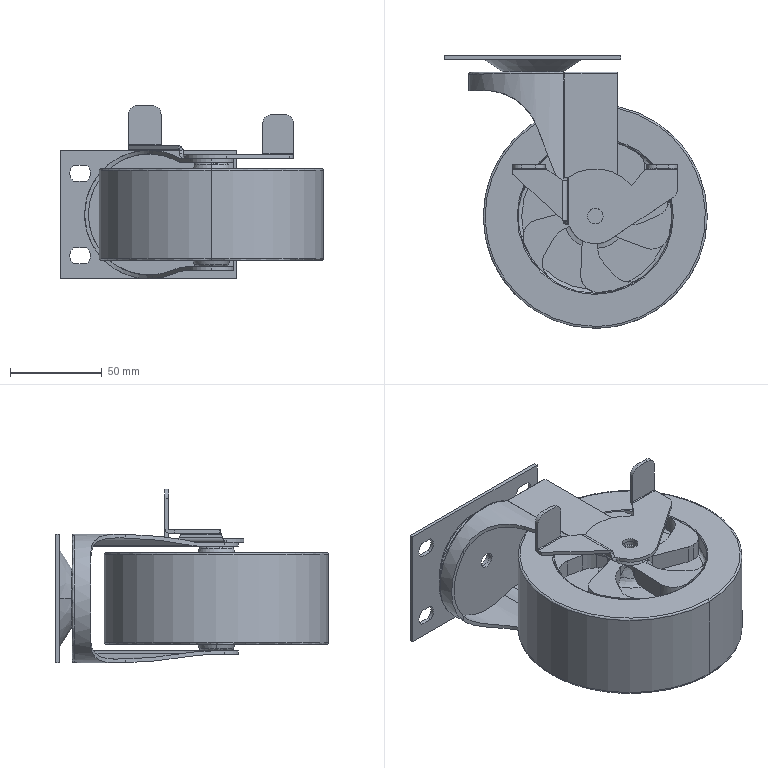Part | SolidWorks | features BaseBody 10, CombineBodies 2 | 4 solids | 281 faces | box 143 x 148.5 x 94.5 mm | volume 569574 mm3 | cylinder 119 | plane 97 | spline 45 | cone 20 | commonest cylinder face diameters 8.5 x14 19.115 x13 11.2 x12 11.664 x12 18.927 x12 26.97 x11